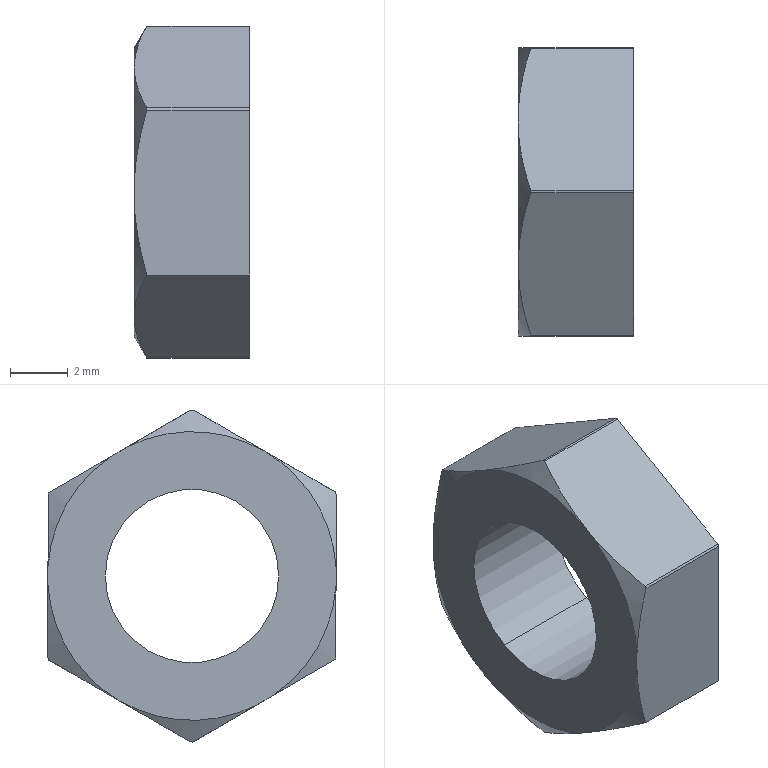Part | STEP file | SANBN6-25-Part-2 | 1 solid | 20 faces | box 4 x 10 x 11.5 mm | volume 231.302 mm3 | plane 8 | cylinder 6 | cone 6 | commonest cylinder face diameters 11.5 x4 6 x2
STEP:
#1=CARTESIAN_POINT('',(8.,1.5,-2.598));
#2=VERTEX_POINT('',#1);
#3=CARTESIAN_POINT('',(8.,-1.5,2.598));
#4=VERTEX_POINT('',#3);
#5=CARTESIAN_POINT('',(8.,0.,0.));
#6=DIRECTION('',(-1.,0.,0.));
#7=DIRECTION('',(0.,-0.5,0.866));
#8=AXIS2_PLACEMENT_3D('',#5,#6,#7);
#9=CIRCLE('',#8,3.);
#10=EDGE_CURVE('',#2,#4,#9,.T.);
#11=ORIENTED_EDGE('',*,*,#10,.T.);
#12=CARTESIAN_POINT('',(12.,-1.5,2.598));
#13=VERTEX_POINT('',#12);
#14=CARTESIAN_POINT('',(30.,-1.5,2.598));
#15=DIRECTION('',(1.,0.,0.));
#16=VECTOR('',#15,1000.);
#17=LINE('',#14,#16);
#18=EDGE_CURVE('',#4,#13,#17,.T.);
#19=ORIENTED_EDGE('',*,*,#18,.T.);
#20=CARTESIAN_POINT('',(12.,1.5,-2.598));
#21=VERTEX_POINT('',#20);
#22=CARTESIAN_POINT('',(12.,0.,0.));
#23=DIRECTION('',(1.,0.,0.));
#24=DIRECTION('',(0.,0.5,-0.866));
#25=AXIS2_PLACEMENT_3D('',#22,#23,#24);
#26=CIRCLE('',#25,3.);
#27=EDGE_CURVE('',#13,#21,#26,.T.);
#28=ORIENTED_EDGE('',*,*,#27,.T.);
#29=CARTESIAN_POINT('',(30.,1.5,-2.598));
#30=DIRECTION('',(1.,0.,0.));
#31=VECTOR('',#30,1000.);
#32=LINE('',#29,#31);
#33=EDGE_CURVE('',#2,#21,#32,.T.);
#34=ORIENTED_EDGE('',*,*,#33,.F.);
#35=EDGE_LOOP('',(#11,#19,#28,#34));
#36=FACE_OUTER_BOUND('',#35,.T.);
#37=CARTESIAN_POINT('',(30.,0.,0.));
#38=DIRECTION('',(1.,0.,0.));
#39=DIRECTION('',(0.,0.5,-0.866));
#40=AXIS2_PLACEMENT_3D('',#37,#38,#39);
#41=CYLINDRICAL_SURFACE('',#40,3.);
#42=ADVANCED_FACE('',(#36),#41,.F.);
#43=CARTESIAN_POINT('',(12.,0.04062,5.75));
#44=VERTEX_POINT('',#43);
#45=CARTESIAN_POINT('',(12.,-0.04096,5.75));
#46=VERTEX_POINT('',#45);
#47=CARTESIAN_POINT('',(12.,0.,0.));
#48=DIRECTION('',(1.,0.,0.));
#49=DIRECTION('',(0.,0.5,-0.866));
#50=AXIS2_PLACEMENT_3D('',#47,#48,#49);
#51=CIRCLE('',#50,5.75);
#52=EDGE_CURVE('',#44,#46,#51,.T.);
#53=ORIENTED_EDGE('',*,*,#52,.F.);
#54=CARTESIAN_POINT('',(8.433,0.04062,5.75));
#55=VERTEX_POINT('',#54);
#56=CARTESIAN_POINT('',(8.,0.04062,5.75));
#57=DIRECTION('',(1.,0.,0.));
#58=VECTOR('',#57,1000.);
#59=LINE('',#56,#58);
#60=EDGE_CURVE('',#55,#44,#59,.T.);
#61=ORIENTED_EDGE('',*,*,#60,.F.);
#62=CARTESIAN_POINT('',(8.433,-0.04096,5.75));
#63=VERTEX_POINT('',#62);
#64=CARTESIAN_POINT('',(8.433,0.,0.));
#65=DIRECTION('',(1.,0.,0.));
#66=DIRECTION('',(0.,0.5,-0.866));
#67=AXIS2_PLACEMENT_3D('',#64,#65,#66);
#68=CIRCLE('',#67,5.75);
#69=EDGE_CURVE('',#55,#63,#68,.T.);
#70=ORIENTED_EDGE('',*,*,#69,.T.);
#71=CARTESIAN_POINT('',(8.,-0.04096,5.75));
#72=DIRECTION('',(-1.,0.,0.));
#73=VECTOR('',#72,1000.);
#74=LINE('',#71,#73);
#75=EDGE_CURVE('',#46,#63,#74,.T.);
#76=ORIENTED_EDGE('',*,*,#75,.F.);
#77=EDGE_LOOP('',(#53,#61,#70,#76));
#78=FACE_OUTER_BOUND('',#77,.T.);
#79=CARTESIAN_POINT('',(8.,0.,0.));
#80=DIRECTION('',(-1.,0.,0.));
#81=DIRECTION('',(0.,0.5,-0.866));
#82=AXIS2_PLACEMENT_3D('',#79,#80,#81);
#83=CYLINDRICAL_SURFACE('',#82,5.75);
#84=ADVANCED_FACE('',(#78),#83,.T.);
#85=CARTESIAN_POINT('',(12.,-0.04062,-5.75));
#86=VERTEX_POINT('',#85);
#87=CARTESIAN_POINT('',(12.,0.04096,-5.75));
#88=VERTEX_POINT('',#87);
#89=CARTESIAN_POINT('',(12.,0.,0.));
#90=DIRECTION('',(1.,0.,0.));
#91=DIRECTION('',(0.,0.5,-0.866));
#92=AXIS2_PLACEMENT_3D('',#89,#90,#91);
#93=CIRCLE('',#92,5.75);
#94=EDGE_CURVE('',#86,#88,#93,.T.);
#95=ORIENTED_EDGE('',*,*,#94,.F.);
#96=CARTESIAN_POINT('',(8.433,-0.04062,-5.75));
#97=VERTEX_POINT('',#96);
#98=CARTESIAN_POINT('',(8.,-0.04062,-5.75));
#99=DIRECTION('',(1.,0.,0.));
#100=VECTOR('',#99,1000.);
#101=LINE('',#98,#100);
#102=EDGE_CURVE('',#97,#86,#101,.T.);
#103=ORIENTED_EDGE('',*,*,#102,.F.);
#104=CARTESIAN_POINT('',(8.433,0.04096,-5.75));
#105=VERTEX_POINT('',#104);
#106=CARTESIAN_POINT('',(8.433,0.,0.));
#107=DIRECTION('',(1.,0.,0.));
#108=DIRECTION('',(0.,0.5,-0.866));
#109=AXIS2_PLACEMENT_3D('',#106,#107,#108);
#110=CIRCLE('',#109,5.75);
#111=EDGE_CURVE('',#97,#105,#110,.T.);
#112=ORIENTED_EDGE('',*,*,#111,.T.);
#113=CARTESIAN_POINT('',(8.,0.04096,-5.75));
#114=DIRECTION('',(-1.,0.,0.));
#115=VECTOR('',#114,1000.);
#116=LINE('',#113,#115);
#117=EDGE_CURVE('',#88,#105,#116,.T.);
#118=ORIENTED_EDGE('',*,*,#117,.F.);
#119=EDGE_LOOP('',(#95,#103,#112,#118));
#120=FACE_OUTER_BOUND('',#119,.T.);
#121=CARTESIAN_POINT('',(8.,0.,0.));
#122=DIRECTION('',(-1.,0.,0.));
#123=DIRECTION('',(0.,0.5,-0.866));
#124=AXIS2_PLACEMENT_3D('',#121,#122,#123);
#125=CYLINDRICAL_SURFACE('',#124,5.75);
#126=ADVANCED_FACE('',(#120),#125,.T.);
#127=CARTESIAN_POINT('',(8.433,-4.959,2.91));
#128=VERTEX_POINT('',#127);
#129=CARTESIAN_POINT('',(8.433,-5.,2.84));
#130=VERTEX_POINT('',#129);
#131=CARTESIAN_POINT('',(8.433,0.,0.));
#132=DIRECTION('',(1.,0.,0.));
#133=DIRECTION('',(0.,0.5,-0.866));
#134=AXIS2_PLACEMENT_3D('',#131,#132,#133);
#135=CIRCLE('',#134,5.75);
#136=EDGE_CURVE('',#128,#130,#135,.T.);
#137=ORIENTED_EDGE('',*,*,#136,.T.);
#138=CARTESIAN_POINT('',(12.,-5.,2.84));
#139=VERTEX_POINT('',#138);
#140=CARTESIAN_POINT('',(8.,-5.,2.84));
#141=DIRECTION('',(-1.,0.,0.));
#142=VECTOR('',#141,1000.);
#143=LINE('',#140,#142);
#144=EDGE_CURVE('',#139,#130,#143,.T.);
#145=ORIENTED_EDGE('',*,*,#144,.F.);
#146=CARTESIAN_POINT('',(12.,-4.959,2.91));
#147=VERTEX_POINT('',#146);
#148=CARTESIAN_POINT('',(12.,0.,0.));
#149=DIRECTION('',(1.,0.,0.));
#150=DIRECTION('',(0.,0.5,-0.866));
#151=AXIS2_PLACEMENT_3D('',#148,#149,#150);
#152=CIRCLE('',#151,5.75);
#153=EDGE_CURVE('',#147,#139,#152,.T.);
#154=ORIENTED_EDGE('',*,*,#153,.F.);
#155=CARTESIAN_POINT('',(8.,-4.959,2.91));
#156=DIRECTION('',(1.,0.,0.));
#157=VECTOR('',#156,1000.);
#158=LINE('',#155,#157);
#159=EDGE_CURVE('',#128,#147,#158,.T.);
#160=ORIENTED_EDGE('',*,*,#159,.F.);
#161=EDGE_LOOP('',(#137,#145,#154,#160));
#162=FACE_OUTER_BOUND('',#161,.T.);
#163=CARTESIAN_POINT('',(8.,0.,0.));
#164=DIRECTION('',(-1.,0.,0.));
#165=DIRECTION('',(0.,0.5,-0.866));
#166=AXIS2_PLACEMENT_3D('',#163,#164,#165);
#167=CYLINDRICAL_SURFACE('',#166,5.75);
#168=ADVANCED_FACE('',(#162),#167,.T.);
#169=ORIENTED_EDGE('',*,*,#69,.F.);
#170=CARTESIAN_POINT('',(8.,2.234,4.473));
#171=VERTEX_POINT('',#170);
#172=CARTESIAN_POINT('',(8.,2.234,4.473));
#173=CARTESIAN_POINT('',(8.032,1.487,4.908));
#174=CARTESIAN_POINT('',(8.195,0.7583,5.332));
#175=CARTESIAN_POINT('',(8.433,0.04062,5.75));
#176=B_SPLINE_CURVE_WITH_KNOTS('',3,(#172,#173,#174,#175),.UNSPECIFIED.,.F.,.F.,(4,4),(0.003207,0.005771),.UNSPECIFIED.);
#177=EDGE_CURVE('',#171,#55,#176,.T.);
#178=ORIENTED_EDGE('',*,*,#177,.F.);
#179=CARTESIAN_POINT('',(8.,-2.5,4.33));
#180=VERTEX_POINT('',#179);
#181=CARTESIAN_POINT('',(8.,0.,0.));
#182=DIRECTION('',(1.,0.,0.));
#183=DIRECTION('',(0.,0.5,-0.866));
#184=AXIS2_PLACEMENT_3D('',#181,#182,#183);
#185=CIRCLE('',#184,5.);
#186=EDGE_CURVE('',#171,#180,#185,.T.);
#187=ORIENTED_EDGE('',*,*,#186,.T.);
#188=CARTESIAN_POINT('',(8.433,-0.04096,5.75));
#189=CARTESIAN_POINT('',(8.169,-0.8423,5.287));
#190=CARTESIAN_POINT('',(8.,-1.658,4.816));
#191=CARTESIAN_POINT('',(8.,-2.5,4.33));
#192=B_SPLINE_CURVE_WITH_KNOTS('',3,(#188,#189,#190,#191),.UNSPECIFIED.,.F.,.F.,(4,4),(0.006338,0.009225),.UNSPECIFIED.);
#193=EDGE_CURVE('',#63,#180,#192,.T.);
#194=ORIENTED_EDGE('',*,*,#193,.F.);
#195=EDGE_LOOP('',(#169,#178,#187,#194));
#196=FACE_OUTER_BOUND('',#195,.T.);
#197=CARTESIAN_POINT('',(8.433,0.,0.));
#198=DIRECTION('',(1.,0.,0.));
#199=DIRECTION('',(0.,-0.5,0.866));
#200=AXIS2_PLACEMENT_3D('',#197,#198,#199);
#201=CONICAL_SURFACE('',#200,5.75,1.047);
#202=ADVANCED_FACE('',(#196),#201,.T.);
#203=CARTESIAN_POINT('',(8.,-4.991,0.302));
#204=VERTEX_POINT('',#203);
#205=CARTESIAN_POINT('',(8.,0.,0.));
#206=DIRECTION('',(1.,0.,0.));
#207=DIRECTION('',(0.,0.5,-0.866));
#208=AXIS2_PLACEMENT_3D('',#205,#206,#207);
#209=CIRCLE('',#208,5.);
#210=EDGE_CURVE('',#180,#204,#209,.T.);
#211=ORIENTED_EDGE('',*,*,#210,.T.);
#212=CARTESIAN_POINT('',(8.433,-5.,2.84));
#213=CARTESIAN_POINT('',(8.194,-4.997,2.007));
#214=CARTESIAN_POINT('',(8.032,-4.994,1.164));
#215=CARTESIAN_POINT('',(8.,-4.991,0.302));
#216=B_SPLINE_CURVE_WITH_KNOTS('',3,(#212,#213,#214,#215),.UNSPECIFIED.,.F.,.F.,(4,4),(0.000002513,0.002576),.UNSPECIFIED.);
#217=EDGE_CURVE('',#130,#204,#216,.T.);
#218=ORIENTED_EDGE('',*,*,#217,.F.);
#219=ORIENTED_EDGE('',*,*,#136,.F.);
#220=CARTESIAN_POINT('',(8.,-2.5,4.33));
#221=CARTESIAN_POINT('',(8.,-2.921,4.087));
#222=CARTESIAN_POINT('',(8.042,-3.336,3.847));
#223=CARTESIAN_POINT('',(8.193,-4.155,3.375));
#224=CARTESIAN_POINT('',(8.301,-4.559,3.141));
#225=CARTESIAN_POINT('',(8.433,-4.959,2.91));
#226=B_SPLINE_CURVE_WITH_KNOTS('',3,(#220,#221,#222,#223,#224,#225),.UNSPECIFIED.,.F.,.F.,(4,2,4),(0.009225,0.01067,0.01211),.UNSPECIFIED.);
#227=EDGE_CURVE('',#180,#128,#226,.T.);
#228=ORIENTED_EDGE('',*,*,#227,.F.);
#229=EDGE_LOOP('',(#211,#218,#219,#228));
#230=FACE_OUTER_BOUND('',#229,.T.);
#231=CARTESIAN_POINT('',(8.433,0.,0.));
#232=DIRECTION('',(1.,0.,0.));
#233=DIRECTION('',(0.,-0.5,0.866));
#234=AXIS2_PLACEMENT_3D('',#231,#232,#233);
#235=CONICAL_SURFACE('',#234,5.75,1.047);
#236=ADVANCED_FACE('',(#230),#235,.T.);
#237=CARTESIAN_POINT('',(8.433,4.959,-2.91));
#238=VERTEX_POINT('',#237);
#239=CARTESIAN_POINT('',(8.433,5.,-2.84));
#240=VERTEX_POINT('',#239);
#241=CARTESIAN_POINT('',(8.433,0.,0.));
#242=DIRECTION('',(1.,0.,0.));
#243=DIRECTION('',(0.,0.5,-0.866));
#244=AXIS2_PLACEMENT_3D('',#241,#242,#243);
#245=CIRCLE('',#244,5.75);
#246=EDGE_CURVE('',#238,#240,#245,.T.);
#247=ORIENTED_EDGE('',*,*,#246,.F.);
#248=CARTESIAN_POINT('',(8.,2.5,-4.33));
#249=VERTEX_POINT('',#248);
#250=CARTESIAN_POINT('',(8.,2.5,-4.33));
#251=CARTESIAN_POINT('',(8.,2.921,-4.087));
#252=CARTESIAN_POINT('',(8.042,3.336,-3.847));
#253=CARTESIAN_POINT('',(8.193,4.155,-3.375));
#254=CARTESIAN_POINT('',(8.301,4.559,-3.141));
#255=CARTESIAN_POINT('',(8.433,4.959,-2.91));
#256=B_SPLINE_CURVE_WITH_KNOTS('',3,(#250,#251,#252,#253,#254,#255),.UNSPECIFIED.,.F.,.F.,(4,2,4),(0.009225,0.01067,0.01211),.UNSPECIFIED.);
#257=EDGE_CURVE('',#249,#238,#256,.T.);
#258=ORIENTED_EDGE('',*,*,#257,.F.);
#259=CARTESIAN_POINT('',(8.,4.991,-0.302));
#260=VERTEX_POINT('',#259);
#261=CARTESIAN_POINT('',(8.,0.,0.));
#262=DIRECTION('',(1.,0.,0.));
#263=DIRECTION('',(0.,0.5,-0.866));
#264=AXIS2_PLACEMENT_3D('',#261,#262,#263);
#265=CIRCLE('',#264,5.);
#266=EDGE_CURVE('',#249,#260,#265,.T.);
#267=ORIENTED_EDGE('',*,*,#266,.T.);
#268=CARTESIAN_POINT('',(8.433,5.,-2.84));
#269=CARTESIAN_POINT('',(8.194,4.997,-2.007));
#270=CARTESIAN_POINT('',(8.032,4.994,-1.164));
#271=CARTESIAN_POINT('',(8.,4.991,-0.302));
#272=B_SPLINE_CURVE_WITH_KNOTS('',3,(#268,#269,#270,#271),.UNSPECIFIED.,.F.,.F.,(4,4),(0.000002513,0.002576),.UNSPECIFIED.);
#273=EDGE_CURVE('',#240,#260,#272,.T.);
#274=ORIENTED_EDGE('',*,*,#273,.F.);
#275=EDGE_LOOP('',(#247,#258,#267,#274));
#276=FACE_OUTER_BOUND('',#275,.T.);
#277=CARTESIAN_POINT('',(8.433,0.,0.));
#278=DIRECTION('',(1.,0.,0.));
#279=DIRECTION('',(0.,-0.5,0.866));
#280=AXIS2_PLACEMENT_3D('',#277,#278,#279);
#281=CONICAL_SURFACE('',#280,5.75,1.047);
#282=ADVANCED_FACE('',(#276),#281,.T.);
#283=ORIENTED_EDGE('',*,*,#111,.F.);
#284=CARTESIAN_POINT('',(8.,-2.234,-4.473));
#285=VERTEX_POINT('',#284);
#286=CARTESIAN_POINT('',(8.,-2.234,-4.473));
#287=CARTESIAN_POINT('',(8.032,-1.487,-4.908));
#288=CARTESIAN_POINT('',(8.195,-0.7583,-5.332));
#289=CARTESIAN_POINT('',(8.433,-0.04062,-5.75));
#290=B_SPLINE_CURVE_WITH_KNOTS('',3,(#286,#287,#288,#289),.UNSPECIFIED.,.F.,.F.,(4,4),(0.003207,0.005771),.UNSPECIFIED.);
#291=EDGE_CURVE('',#285,#97,#290,.T.);
#292=ORIENTED_EDGE('',*,*,#291,.F.);
#293=CARTESIAN_POINT('',(8.,0.,0.));
#294=DIRECTION('',(1.,0.,0.));
#295=DIRECTION('',(0.,0.5,-0.866));
#296=AXIS2_PLACEMENT_3D('',#293,#294,#295);
#297=CIRCLE('',#296,5.);
#298=EDGE_CURVE('',#285,#249,#297,.T.);
#299=ORIENTED_EDGE('',*,*,#298,.T.);
#300=CARTESIAN_POINT('',(8.433,0.04096,-5.75));
#301=CARTESIAN_POINT('',(8.169,0.8423,-5.287));
#302=CARTESIAN_POINT('',(8.,1.658,-4.816));
#303=CARTESIAN_POINT('',(8.,2.5,-4.33));
#304=B_SPLINE_CURVE_WITH_KNOTS('',3,(#300,#301,#302,#303),.UNSPECIFIED.,.F.,.F.,(4,4),(0.006338,0.009225),.UNSPECIFIED.);
#305=EDGE_CURVE('',#105,#249,#304,.T.);
#306=ORIENTED_EDGE('',*,*,#305,.F.);
#307=EDGE_LOOP('',(#283,#292,#299,#306));
#308=FACE_OUTER_BOUND('',#307,.T.);
#309=CARTESIAN_POINT('',(8.433,0.,0.));
#310=DIRECTION('',(1.,0.,0.));
#311=DIRECTION('',(0.,-0.5,0.866));
#312=AXIS2_PLACEMENT_3D('',#309,#310,#311);
#313=CONICAL_SURFACE('',#312,5.75,1.047);
#314=ADVANCED_FACE('',(#308),#313,.T.);
#315=CARTESIAN_POINT('',(8.,4.989,0.3373));
#316=VERTEX_POINT('',#315);
#317=CARTESIAN_POINT('',(8.,2.786,4.152));
#318=VERTEX_POINT('',#317);
#319=CARTESIAN_POINT('',(8.,0.,0.));
#320=DIRECTION('',(1.,0.,0.));
#321=DIRECTION('',(0.,0.5,-0.866));
#322=AXIS2_PLACEMENT_3D('',#319,#320,#321);
#323=CIRCLE('',#322,5.);
#324=EDGE_CURVE('',#316,#318,#323,.T.);
#325=ORIENTED_EDGE('',*,*,#324,.T.);
#326=CARTESIAN_POINT('',(8.433,4.98,2.875));
#327=VERTEX_POINT('',#326);
#328=CARTESIAN_POINT('',(8.433,4.98,2.875));
#329=CARTESIAN_POINT('',(8.194,4.26,3.294));
#330=CARTESIAN_POINT('',(8.032,3.531,3.718));
#331=CARTESIAN_POINT('',(8.,2.786,4.152));
#332=B_SPLINE_CURVE_WITH_KNOTS('',3,(#328,#329,#330,#331),.UNSPECIFIED.,.F.,.F.,(4,4),(0.000000831,0.002574),.UNSPECIFIED.);
#333=EDGE_CURVE('',#327,#318,#332,.T.);
#334=ORIENTED_EDGE('',*,*,#333,.F.);
#335=CARTESIAN_POINT('',(8.,4.989,0.3373));
#336=CARTESIAN_POINT('',(8.032,4.986,1.202));
#337=CARTESIAN_POINT('',(8.195,4.983,2.045));
#338=CARTESIAN_POINT('',(8.433,4.98,2.875));
#339=B_SPLINE_CURVE_WITH_KNOTS('',3,(#335,#336,#337,#338),.UNSPECIFIED.,.F.,.F.,(4,4),(0.003209,0.005772),.UNSPECIFIED.);
#340=EDGE_CURVE('',#316,#327,#339,.T.);
#341=ORIENTED_EDGE('',*,*,#340,.F.);
#342=EDGE_LOOP('',(#325,#334,#341));
#343=FACE_OUTER_BOUND('',#342,.T.);
#344=CARTESIAN_POINT('',(8.433,0.,0.));
#345=DIRECTION('',(1.,0.,0.));
#346=DIRECTION('',(0.,-0.5,0.866));
#347=AXIS2_PLACEMENT_3D('',#344,#345,#346);
#348=CONICAL_SURFACE('',#347,5.75,1.047);
#349=ADVANCED_FACE('',(#343),#348,.T.);
#350=CARTESIAN_POINT('',(12.,4.98,2.875));
#351=VERTEX_POINT('',#350);
#352=CARTESIAN_POINT('',(12.,4.98,2.875));
#353=DIRECTION('',(0.,-0.8643,0.5031));
#354=VECTOR('',#353,1000.);
#355=LINE('',#352,#354);
#356=EDGE_CURVE('',#351,#44,#355,.T.);
#357=ORIENTED_EDGE('',*,*,#356,.T.);
#358=ORIENTED_EDGE('',*,*,#52,.T.);
#359=CARTESIAN_POINT('',(12.,0.,5.774));
#360=DIRECTION('',(0.,-0.866,-0.5));
#361=VECTOR('',#360,1000.);
#362=LINE('',#359,#361);
#363=EDGE_CURVE('',#46,#147,#362,.T.);
#364=ORIENTED_EDGE('',*,*,#363,.T.);
#365=ORIENTED_EDGE('',*,*,#153,.T.);
#366=CARTESIAN_POINT('',(12.,-4.98,-2.875));
#367=VERTEX_POINT('',#366);
#368=CARTESIAN_POINT('',(12.,-5.,2.887));
#369=DIRECTION('',(0.,0.003533,-1.));
#370=VECTOR('',#369,1000.);
#371=LINE('',#368,#370);
#372=EDGE_CURVE('',#139,#367,#371,.T.);
#373=ORIENTED_EDGE('',*,*,#372,.T.);
#374=CARTESIAN_POINT('',(12.,-4.98,-2.875));
#375=DIRECTION('',(0.,0.8643,-0.5031));
#376=VECTOR('',#375,1000.);
#377=LINE('',#374,#376);
#378=EDGE_CURVE('',#367,#86,#377,.T.);
#379=ORIENTED_EDGE('',*,*,#378,.T.);
#380=ORIENTED_EDGE('',*,*,#94,.T.);
#381=CARTESIAN_POINT('',(12.,4.959,-2.91));
#382=VERTEX_POINT('',#381);
#383=CARTESIAN_POINT('',(12.,0.,-5.774));
#384=DIRECTION('',(0.,0.866,0.5));
#385=VECTOR('',#384,1000.);
#386=LINE('',#383,#385);
#387=EDGE_CURVE('',#88,#382,#386,.T.);
#388=ORIENTED_EDGE('',*,*,#387,.T.);
#389=CARTESIAN_POINT('',(12.,5.,-2.84));
#390=VERTEX_POINT('',#389);
#391=CARTESIAN_POINT('',(12.,0.,0.));
#392=DIRECTION('',(1.,0.,0.));
#393=DIRECTION('',(0.,0.5,-0.866));
#394=AXIS2_PLACEMENT_3D('',#391,#392,#393);
#395=CIRCLE('',#394,5.75);
#396=EDGE_CURVE('',#382,#390,#395,.T.);
#397=ORIENTED_EDGE('',*,*,#396,.T.);
#398=CARTESIAN_POINT('',(12.,5.,-2.887));
#399=DIRECTION('',(0.,-0.003533,1.));
#400=VECTOR('',#399,1000.);
#401=LINE('',#398,#400);
#402=EDGE_CURVE('',#390,#351,#401,.T.);
#403=ORIENTED_EDGE('',*,*,#402,.T.);
#404=EDGE_LOOP('',(#357,#358,#364,#365,#373,#379,#380,#388,#397,#403));
#405=FACE_OUTER_BOUND('',#404,.T.);
#406=CARTESIAN_POINT('',(12.,0.,0.));
#407=DIRECTION('',(1.,0.,0.));
#408=DIRECTION('',(0.,0.5,-0.866));
#409=AXIS2_PLACEMENT_3D('',#406,#407,#408);
#410=CIRCLE('',#409,3.);
#411=EDGE_CURVE('',#21,#13,#410,.T.);
#412=ORIENTED_EDGE('',*,*,#411,.F.);
#413=ORIENTED_EDGE('',*,*,#27,.F.);
#414=EDGE_LOOP('',(#412,#413));
#415=FACE_BOUND('',#414,.T.);
#416=CARTESIAN_POINT('',(12.,0.,0.));
#417=DIRECTION('',(-1.,0.,0.));
#418=DIRECTION('',(0.,0.5,-0.866));
#419=AXIS2_PLACEMENT_3D('',#416,#417,#418);
#420=PLANE('',#419);
#421=ADVANCED_FACE('',(#405,#415),#420,.F.);
#422=ORIENTED_EDGE('',*,*,#396,.F.);
#423=CARTESIAN_POINT('',(8.,4.959,-2.91));
#424=DIRECTION('',(1.,0.,0.));
#425=VECTOR('',#424,1000.);
#426=LINE('',#423,#425);
#427=EDGE_CURVE('',#238,#382,#426,.T.);
#428=ORIENTED_EDGE('',*,*,#427,.F.);
#429=ORIENTED_EDGE('',*,*,#246,.T.);
#430=CARTESIAN_POINT('',(8.,5.,-2.84));
#431=DIRECTION('',(-1.,0.,0.));
#432=VECTOR('',#431,1000.);
#433=LINE('',#430,#432);
#434=EDGE_CURVE('',#390,#240,#433,.T.);
#435=ORIENTED_EDGE('',*,*,#434,.F.);
#436=EDGE_LOOP('',(#422,#428,#429,#435));
#437=FACE_OUTER_BOUND('',#436,.T.);
#438=CARTESIAN_POINT('',(8.,0.,0.));
#439=DIRECTION('',(-1.,0.,0.));
#440=DIRECTION('',(0.,0.5,-0.866));
#441=AXIS2_PLACEMENT_3D('',#438,#439,#440);
#442=CYLINDRICAL_SURFACE('',#441,5.75);
#443=ADVANCED_FACE('',(#437),#442,.T.);
#444=CARTESIAN_POINT('',(8.,-4.989,-0.3373));
#445=VERTEX_POINT('',#444);
#446=CARTESIAN_POINT('',(8.433,-4.98,-2.875));
#447=VERTEX_POINT('',#446);
#448=CARTESIAN_POINT('',(8.,-4.989,-0.3373));
#449=CARTESIAN_POINT('',(8.032,-4.986,-1.202));
#450=CARTESIAN_POINT('',(8.195,-4.983,-2.045));
#451=CARTESIAN_POINT('',(8.433,-4.98,-2.875));
#452=B_SPLINE_CURVE_WITH_KNOTS('',3,(#448,#449,#450,#451),.UNSPECIFIED.,.F.,.F.,(4,4),(0.003209,0.005772),.UNSPECIFIED.);
#453=EDGE_CURVE('',#445,#447,#452,.T.);
#454=ORIENTED_EDGE('',*,*,#453,.F.);
#455=CARTESIAN_POINT('',(8.,-2.786,-4.152));
#456=VERTEX_POINT('',#455);
#457=CARTESIAN_POINT('',(8.,0.,0.));
#458=DIRECTION('',(1.,0.,0.));
#459=DIRECTION('',(0.,0.5,-0.866));
#460=AXIS2_PLACEMENT_3D('',#457,#458,#459);
#461=CIRCLE('',#460,5.);
#462=EDGE_CURVE('',#445,#456,#461,.T.);
#463=ORIENTED_EDGE('',*,*,#462,.T.);
#464=CARTESIAN_POINT('',(8.433,-4.98,-2.875));
#465=CARTESIAN_POINT('',(8.194,-4.26,-3.294));
#466=CARTESIAN_POINT('',(8.032,-3.531,-3.718));
#467=CARTESIAN_POINT('',(8.,-2.786,-4.152));
#468=B_SPLINE_CURVE_WITH_KNOTS('',3,(#464,#465,#466,#467),.UNSPECIFIED.,.F.,.F.,(4,4),(0.000000831,0.002574),.UNSPECIFIED.);
#469=EDGE_CURVE('',#447,#456,#468,.T.);
#470=ORIENTED_EDGE('',*,*,#469,.F.);
#471=EDGE_LOOP('',(#454,#463,#470));
#472=FACE_OUTER_BOUND('',#471,.T.);
#473=CARTESIAN_POINT('',(8.433,0.,0.));
#474=DIRECTION('',(1.,0.,0.));
#475=DIRECTION('',(0.,-0.5,0.866));
#476=AXIS2_PLACEMENT_3D('',#473,#474,#475);
#477=CONICAL_SURFACE('',#476,5.75,1.047);
#478=ADVANCED_FACE('',(#472),#477,.T.);
#479=ORIENTED_EDGE('',*,*,#10,.F.);
#480=CARTESIAN_POINT('',(8.,0.,0.));
#481=DIRECTION('',(-1.,0.,0.));
#482=DIRECTION('',(0.,-0.5,0.866));
#483=AXIS2_PLACEMENT_3D('',#480,#481,#482);
#484=CIRCLE('',#483,3.);
#485=EDGE_CURVE('',#4,#2,#484,.T.);
#486=ORIENTED_EDGE('',*,*,#485,.F.);
#487=EDGE_LOOP('',(#479,#486));
#488=FACE_BOUND('',#487,.T.);
#489=CARTESIAN_POINT('',(8.,4.981,2.502));
#490=DIRECTION('',(0.,-0.003533,1.));
#491=VECTOR('',#490,1000.);
#492=LINE('',#489,#491);
#493=EDGE_CURVE('',#260,#316,#492,.T.);
#494=ORIENTED_EDGE('',*,*,#493,.F.);
#495=ORIENTED_EDGE('',*,*,#266,.F.);
#496=ORIENTED_EDGE('',*,*,#298,.F.);
#497=CARTESIAN_POINT('',(8.,-0.3627,-5.562));
#498=DIRECTION('',(0.,0.8643,-0.5031));
#499=VECTOR('',#498,1000.);
#500=LINE('',#497,#499);
#501=EDGE_CURVE('',#456,#285,#500,.T.);
#502=ORIENTED_EDGE('',*,*,#501,.F.);
#503=ORIENTED_EDGE('',*,*,#462,.F.);
#504=CARTESIAN_POINT('',(8.,-4.999,2.467));
#505=DIRECTION('',(0.,0.003533,-1.));
#506=VECTOR('',#505,1000.);
#507=LINE('',#504,#506);
#508=EDGE_CURVE('',#204,#445,#507,.T.);
#509=ORIENTED_EDGE('',*,*,#508,.F.);
#510=ORIENTED_EDGE('',*,*,#210,.F.);
#511=ORIENTED_EDGE('',*,*,#186,.F.);
#512=CARTESIAN_POINT('',(8.,4.658,3.062));
#513=DIRECTION('',(0.,-0.8643,0.5031));
#514=VECTOR('',#513,1000.);
#515=LINE('',#512,#514);
#516=EDGE_CURVE('',#318,#171,#515,.T.);
#517=ORIENTED_EDGE('',*,*,#516,.F.);
#518=ORIENTED_EDGE('',*,*,#324,.F.);
#519=EDGE_LOOP('',(#494,#495,#496,#502,#503,#509,#510,#511,#517,#518));
#520=FACE_OUTER_BOUND('',#519,.T.);
#521=CARTESIAN_POINT('',(8.,4.33,2.5));
#522=DIRECTION('',(1.,0.,0.));
#523=DIRECTION('',(0.,-0.5,0.866));
#524=AXIS2_PLACEMENT_3D('',#521,#522,#523);
#525=PLANE('',#524);
#526=ADVANCED_FACE('',(#488,#520),#525,.F.);
#527=ORIENTED_EDGE('',*,*,#372,.F.);
#528=ORIENTED_EDGE('',*,*,#144,.T.);
#529=ORIENTED_EDGE('',*,*,#217,.T.);
#530=ORIENTED_EDGE('',*,*,#508,.T.);
#531=ORIENTED_EDGE('',*,*,#453,.T.);
#532=CARTESIAN_POINT('',(8.,-4.98,-2.875));
#533=DIRECTION('',(1.,0.,0.));
#534=VECTOR('',#533,1000.);
#535=LINE('',#532,#534);
#536=EDGE_CURVE('',#447,#367,#535,.T.);
#537=ORIENTED_EDGE('',*,*,#536,.T.);
#538=EDGE_LOOP('',(#527,#528,#529,#530,#531,#537));
#539=FACE_OUTER_BOUND('',#538,.T.);
#540=CARTESIAN_POINT('',(8.,-5.,2.887));
#541=DIRECTION('',(0.,1.,0.003533));
#542=DIRECTION('',(0.,-0.003533,1.));
#543=AXIS2_PLACEMENT_3D('',#540,#541,#542);
#544=PLANE('',#543);
#545=ADVANCED_FACE('',(#539),#544,.F.);
#546=ORIENTED_EDGE('',*,*,#536,.F.);
#547=ORIENTED_EDGE('',*,*,#469,.T.);
#548=ORIENTED_EDGE('',*,*,#501,.T.);
#549=ORIENTED_EDGE('',*,*,#291,.T.);
#550=ORIENTED_EDGE('',*,*,#102,.T.);
#551=ORIENTED_EDGE('',*,*,#378,.F.);
#552=EDGE_LOOP('',(#546,#547,#548,#549,#550,#551));
#553=FACE_OUTER_BOUND('',#552,.T.);
#554=CARTESIAN_POINT('',(8.,-4.98,-2.875));
#555=DIRECTION('',(0.,0.5031,0.8643));
#556=DIRECTION('',(0.,-0.8643,0.5031));
#557=AXIS2_PLACEMENT_3D('',#554,#555,#556);
#558=PLANE('',#557);
#559=ADVANCED_FACE('',(#553),#558,.F.);
#560=ORIENTED_EDGE('',*,*,#402,.F.);
#561=ORIENTED_EDGE('',*,*,#434,.T.);
#562=ORIENTED_EDGE('',*,*,#273,.T.);
#563=ORIENTED_EDGE('',*,*,#493,.T.);
#564=ORIENTED_EDGE('',*,*,#340,.T.);
#565=CARTESIAN_POINT('',(8.,4.98,2.875));
#566=DIRECTION('',(1.,0.,0.));
#567=VECTOR('',#566,1000.);
#568=LINE('',#565,#567);
#569=EDGE_CURVE('',#327,#351,#568,.T.);
#570=ORIENTED_EDGE('',*,*,#569,.T.);
#571=EDGE_LOOP('',(#560,#561,#562,#563,#564,#570));
#572=FACE_OUTER_BOUND('',#571,.T.);
#573=CARTESIAN_POINT('',(8.,5.,-2.887));
#574=DIRECTION('',(0.,-1.,-0.003533));
#575=DIRECTION('',(0.,0.003533,-1.));
#576=AXIS2_PLACEMENT_3D('',#573,#574,#575);
#577=PLANE('',#576);
#578=ADVANCED_FACE('',(#572),#577,.F.);
#579=ORIENTED_EDGE('',*,*,#569,.F.);
#580=ORIENTED_EDGE('',*,*,#333,.T.);
#581=ORIENTED_EDGE('',*,*,#516,.T.);
#582=ORIENTED_EDGE('',*,*,#177,.T.);
#583=ORIENTED_EDGE('',*,*,#60,.T.);
#584=ORIENTED_EDGE('',*,*,#356,.F.);
#585=EDGE_LOOP('',(#579,#580,#581,#582,#583,#584));
#586=FACE_OUTER_BOUND('',#585,.T.);
#587=CARTESIAN_POINT('',(8.,4.98,2.875));
#588=DIRECTION('',(0.,-0.5031,-0.8643));
#589=DIRECTION('',(0.,0.8643,-0.5031));
#590=AXIS2_PLACEMENT_3D('',#587,#588,#589);
#591=PLANE('',#590);
#592=ADVANCED_FACE('',(#586),#591,.F.);
#593=ORIENTED_EDGE('',*,*,#387,.F.);
#594=ORIENTED_EDGE('',*,*,#117,.T.);
#595=ORIENTED_EDGE('',*,*,#305,.T.);
#596=ORIENTED_EDGE('',*,*,#257,.T.);
#597=ORIENTED_EDGE('',*,*,#427,.T.);
#598=EDGE_LOOP('',(#593,#594,#595,#596,#597));
#599=FACE_OUTER_BOUND('',#598,.T.);
#600=CARTESIAN_POINT('',(8.,0.,-5.774));
#601=DIRECTION('',(0.,-0.5,0.866));
#602=DIRECTION('',(-1.,0.,0.));
#603=AXIS2_PLACEMENT_3D('',#600,#601,#602);
#604=PLANE('',#603);
#605=ADVANCED_FACE('',(#599),#604,.F.);
#606=ORIENTED_EDGE('',*,*,#363,.F.);
#607=ORIENTED_EDGE('',*,*,#75,.T.);
#608=ORIENTED_EDGE('',*,*,#193,.T.);
#609=ORIENTED_EDGE('',*,*,#227,.T.);
#610=ORIENTED_EDGE('',*,*,#159,.T.);
#611=EDGE_LOOP('',(#606,#607,#608,#609,#610));
#612=FACE_OUTER_BOUND('',#611,.T.);
#613=CARTESIAN_POINT('',(8.,0.,5.774));
#614=DIRECTION('',(0.,0.5,-0.866));
#615=DIRECTION('',(1.,0.,0.));
#616=AXIS2_PLACEMENT_3D('',#613,#614,#615);
#617=PLANE('',#616);
#618=ADVANCED_FACE('',(#612),#617,.F.);
#619=ORIENTED_EDGE('',*,*,#18,.F.);
#620=ORIENTED_EDGE('',*,*,#485,.T.);
#621=ORIENTED_EDGE('',*,*,#33,.T.);
#622=ORIENTED_EDGE('',*,*,#411,.T.);
#623=EDGE_LOOP('',(#619,#620,#621,#622));
#624=FACE_OUTER_BOUND('',#623,.T.);
#625=CARTESIAN_POINT('',(30.,0.,0.));
#626=DIRECTION('',(1.,0.,0.));
#627=DIRECTION('',(0.,0.5,-0.866));
#628=AXIS2_PLACEMENT_3D('',#625,#626,#627);
#629=CYLINDRICAL_SURFACE('',#628,3.);
#630=ADVANCED_FACE('',(#624),#629,.F.);
#631=CLOSED_SHELL('',(#42,#84,#126,#168,#202,#236,#282,#314,#349,#421,#443,#478,#526,#545,#559,#578,#592,#605,#618,#630));
#632=MANIFOLD_SOLID_BREP('',#631);
#633=CARTESIAN_POINT('',(0.,0.,0.));
#634=DIRECTION('',(0.,0.,1.));
#635=DIRECTION('',(1.,0.,0.));
#636=AXIS2_PLACEMENT_3D('',#633,#634,#635);
#637=(LENGTH_UNIT()NAMED_UNIT(*)SI_UNIT(.MILLI.,.METRE.));
#638=UNCERTAINTY_MEASURE_WITH_UNIT(LENGTH_MEASURE(0.00001),#637,'','');
#639=(NAMED_UNIT(*)PLANE_ANGLE_UNIT()SI_UNIT($,.RADIAN.));
#640=(NAMED_UNIT(*)SI_UNIT($,.STERADIAN.)SOLID_ANGLE_UNIT());
#641=(GEOMETRIC_REPRESENTATION_CONTEXT(3)GLOBAL_UNCERTAINTY_ASSIGNED_CONTEXT((#638))GLOBAL_UNIT_ASSIGNED_CONTEXT((#637,#639,#640))REPRESENTATION_CONTEXT('',''));
#642=ADVANCED_BREP_SHAPE_REPRESENTATION('',(#632,#636),#641);